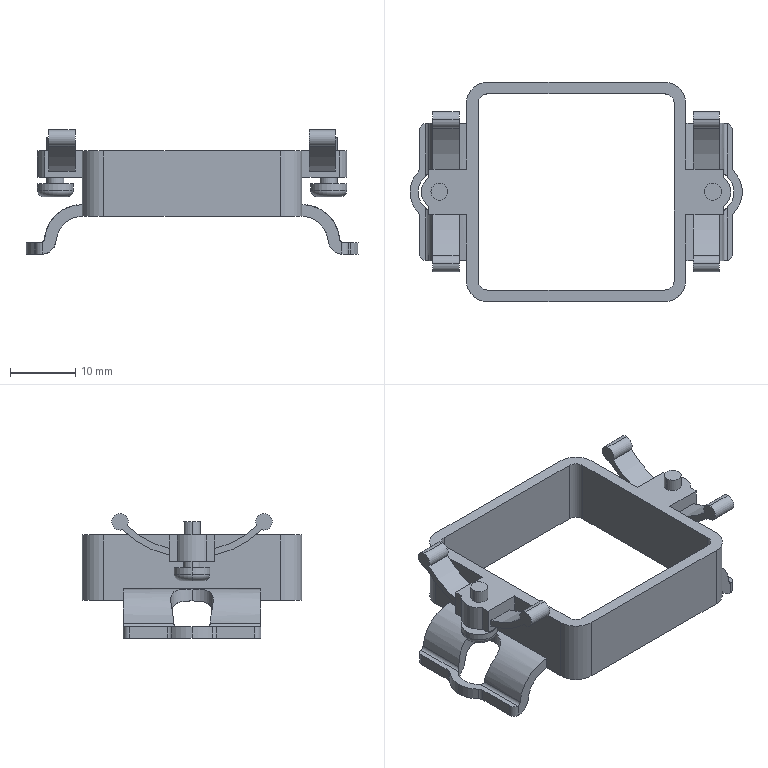Part | SolidWorks | features BaseBody 1 | 1 solid | 120 faces | box 50.8 x 33.6 x 19.05 mm | volume 3493 mm3 | cylinder 70 | plane 46 | torus 4 | commonest cylinder face diameters 2.5 x12 2 x8 2.6 x8 5.5 x7 1 x4 3 x4